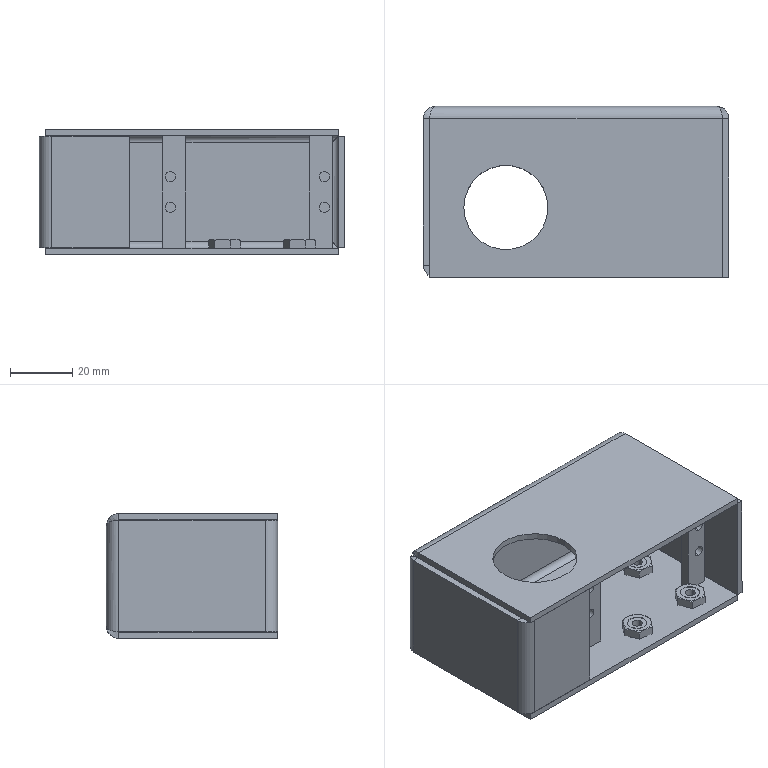Part | SolidWorks | features EdgeFlange 3, CornerFeat 2, ICE 2, LPattern 2, FlatPattern 1, HoleWzd 1, MirrorSolid 1, MoveCopyBody 1, SMBaseFlange 1, SheetMetal 1, Stock 1 | 7 solids | 190 faces | box 98 x 55 x 40 mm | volume 36160 mm3 | plane 104 | cylinder 54 | cone 24 | spline 8 | commonest cylinder face diameters 3.242 x8 3.3 x8 5.97 x8 6 x8 6.18 x8 4 x5